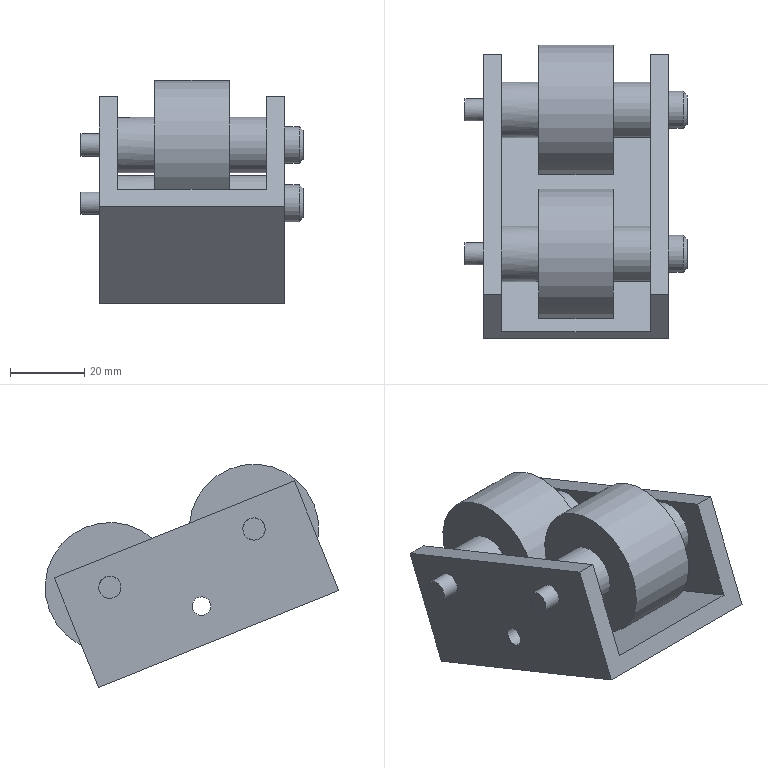Part | NX | features solid 2 | 1 solid | 32 faces | box 60 x 79.34 x 60.356 mm | volume 82796 mm3 | plane 18 | cylinder 12 | cone 2 | commonest cylinder face diameters 15 x4 5 x2 6 x2 10 x2 35 x2
STEP:
#1=CARTESIAN_POINT('',(-651.881,525.03,-99.486));
#2=VERTEX_POINT('',#1);
#3=CARTESIAN_POINT('',(-691.881,525.03,-99.486));
#4=VERTEX_POINT('',#3);
#5=CARTESIAN_POINT('',(-646.881,525.03,-99.486));
#6=DIRECTION('',(-1.,0.,0.));
#7=VECTOR('',#6,1000.);
#8=LINE('',#5,#7);
#9=EDGE_CURVE('',#2,#4,#8,.T.);
#10=ORIENTED_EDGE('',*,*,#9,.F.);
#11=CARTESIAN_POINT('',(-651.881,535.144,-74.452));
#12=VERTEX_POINT('',#11);
#13=CARTESIAN_POINT('',(-651.881,535.144,-74.452));
#14=DIRECTION('',(0.,-0.3746,-0.9272));
#15=VECTOR('',#14,1000.);
#16=LINE('',#13,#15);
#17=EDGE_CURVE('',#12,#2,#16,.T.);
#18=ORIENTED_EDGE('',*,*,#17,.F.);
#19=CARTESIAN_POINT('',(-646.881,535.144,-74.452));
#20=VERTEX_POINT('',#19);
#21=CARTESIAN_POINT('',(-646.881,535.144,-74.452));
#22=DIRECTION('',(-1.,0.,0.));
#23=VECTOR('',#22,1000.);
#24=LINE('',#21,#23);
#25=EDGE_CURVE('',#12,#20,#24,.F.);
#26=ORIENTED_EDGE('',*,*,#25,.T.);
#27=CARTESIAN_POINT('',(-646.881,523.157,-104.122));
#28=VERTEX_POINT('',#27);
#29=CARTESIAN_POINT('',(-646.881,535.144,-74.452));
#30=DIRECTION('',(0.,-0.3746,-0.9272));
#31=VECTOR('',#30,1000.);
#32=LINE('',#29,#31);
#33=EDGE_CURVE('',#20,#28,#32,.T.);
#34=ORIENTED_EDGE('',*,*,#33,.T.);
#35=CARTESIAN_POINT('',(-696.881,523.157,-104.122));
#36=VERTEX_POINT('',#35);
#37=CARTESIAN_POINT('',(-646.881,523.157,-104.122));
#38=DIRECTION('',(-1.,0.,0.));
#39=VECTOR('',#38,1000.);
#40=LINE('',#37,#39);
#41=EDGE_CURVE('',#28,#36,#40,.T.);
#42=ORIENTED_EDGE('',*,*,#41,.T.);
#43=CARTESIAN_POINT('',(-696.881,535.144,-74.452));
#44=VERTEX_POINT('',#43);
#45=CARTESIAN_POINT('',(-696.881,523.157,-104.122));
#46=DIRECTION('',(0.,0.3746,0.9272));
#47=VECTOR('',#46,1000.);
#48=LINE('',#45,#47);
#49=EDGE_CURVE('',#36,#44,#48,.T.);
#50=ORIENTED_EDGE('',*,*,#49,.T.);
#51=CARTESIAN_POINT('',(-691.881,535.144,-74.452));
#52=VERTEX_POINT('',#51);
#53=CARTESIAN_POINT('',(-696.881,535.144,-74.452));
#54=DIRECTION('',(1.,0.,0.));
#55=VECTOR('',#54,1000.);
#56=LINE('',#53,#55);
#57=EDGE_CURVE('',#44,#52,#56,.T.);
#58=ORIENTED_EDGE('',*,*,#57,.T.);
#59=CARTESIAN_POINT('',(-691.881,523.157,-104.122));
#60=DIRECTION('',(0.,0.3746,0.9272));
#61=VECTOR('',#60,1000.);
#62=LINE('',#59,#61);
#63=EDGE_CURVE('',#4,#52,#62,.T.);
#64=ORIENTED_EDGE('',*,*,#63,.F.);
#65=EDGE_LOOP('',(#10,#18,#26,#34,#42,#50,#58,#64));
#66=FACE_BOUND('',#65,.T.);
#67=CARTESIAN_POINT('',(-646.881,535.144,-74.452));
#68=DIRECTION('',(0.,-0.9272,0.3746));
#69=DIRECTION('',(0.,-0.3746,-0.9272));
#70=AXIS2_PLACEMENT_3D('',#67,#68,#69);
#71=PLANE('',#70);
#72=ADVANCED_FACE('',(#66),#71,.F.);
#73=CARTESIAN_POINT('',(-691.881,483.962,-54.313));
#74=VERTEX_POINT('',#73);
#75=CARTESIAN_POINT('',(-691.881,481.152,-61.267));
#76=DIRECTION('',(-1.,0.,0.));
#77=DIRECTION('',(0.,0.3746,0.9272));
#78=AXIS2_PLACEMENT_3D('',#75,#76,#77);
#79=CIRCLE('',#78,7.5);
#80=EDGE_CURVE('',#74,#74,#79,.F.);
#81=ORIENTED_EDGE('',*,*,#80,.F.);
#82=EDGE_LOOP('',(#81));
#83=FACE_BOUND('',#82,.T.);
#84=CARTESIAN_POINT('',(-691.881,460.127,-73.264));
#85=VERTEX_POINT('',#84);
#86=CARTESIAN_POINT('',(-691.881,460.127,-73.264));
#87=DIRECTION('',(0.,0.9272,-0.3746));
#88=VECTOR('',#87,1000.);
#89=LINE('',#86,#88);
#90=EDGE_CURVE('',#85,#4,#89,.T.);
#91=ORIENTED_EDGE('',*,*,#90,.T.);
#92=ORIENTED_EDGE('',*,*,#63,.T.);
#93=CARTESIAN_POINT('',(-691.881,470.241,-48.23));
#94=VERTEX_POINT('',#93);
#95=CARTESIAN_POINT('',(-691.881,470.241,-48.23));
#96=DIRECTION('',(0.,0.9272,-0.3746));
#97=VECTOR('',#96,1000.);
#98=LINE('',#95,#97);
#99=EDGE_CURVE('',#94,#52,#98,.T.);
#100=ORIENTED_EDGE('',*,*,#99,.F.);
#101=CARTESIAN_POINT('',(-691.881,458.254,-77.9));
#102=DIRECTION('',(0.,0.3746,0.9272));
#103=VECTOR('',#102,1000.);
#104=LINE('',#101,#103);
#105=EDGE_CURVE('',#85,#94,#104,.T.);
#106=ORIENTED_EDGE('',*,*,#105,.F.);
#107=EDGE_LOOP('',(#91,#92,#100,#106));
#108=FACE_BOUND('',#107,.T.);
#109=CARTESIAN_POINT('',(-691.881,496.315,-79.796));
#110=VERTEX_POINT('',#109);
#111=CARTESIAN_POINT('',(-691.881,495.379,-82.114));
#112=DIRECTION('',(-1.,0.,0.));
#113=DIRECTION('',(0.,0.3746,0.9272));
#114=AXIS2_PLACEMENT_3D('',#111,#112,#113);
#115=CIRCLE('',#114,2.5);
#116=EDGE_CURVE('',#110,#110,#115,.F.);
#117=ORIENTED_EDGE('',*,*,#116,.F.);
#118=EDGE_LOOP('',(#117));
#119=FACE_BOUND('',#118,.T.);
#120=CARTESIAN_POINT('',(-691.881,522.904,-70.046));
#121=VERTEX_POINT('',#120);
#122=CARTESIAN_POINT('',(-691.881,520.094,-77.));
#123=DIRECTION('',(-1.,0.,0.));
#124=DIRECTION('',(0.,0.3746,0.9272));
#125=AXIS2_PLACEMENT_3D('',#122,#123,#124);
#126=CIRCLE('',#125,7.5);
#127=EDGE_CURVE('',#121,#121,#126,.F.);
#128=ORIENTED_EDGE('',*,*,#127,.F.);
#129=EDGE_LOOP('',(#128));
#130=FACE_BOUND('',#129,.T.);
#131=CARTESIAN_POINT('',(-691.881,458.254,-77.9));
#132=DIRECTION('',(-1.,0.,0.));
#133=DIRECTION('',(0.,0.3746,0.9272));
#134=AXIS2_PLACEMENT_3D('',#131,#132,#133);
#135=PLANE('',#134);
#136=ADVANCED_FACE('',(#83,#108,#119,#130),#135,.F.);
#137=CARTESIAN_POINT('',(-651.881,527.048,-79.81));
#138=VERTEX_POINT('',#137);
#139=CARTESIAN_POINT('',(-651.881,520.094,-77.));
#140=DIRECTION('',(-1.,0.,0.));
#141=DIRECTION('',(0.,0.9272,-0.3746));
#142=AXIS2_PLACEMENT_3D('',#139,#140,#141);
#143=CIRCLE('',#142,7.5);
#144=EDGE_CURVE('',#138,#138,#143,.T.);
#145=ORIENTED_EDGE('',*,*,#144,.F.);
#146=EDGE_LOOP('',(#145));
#147=FACE_BOUND('',#146,.T.);
#148=CARTESIAN_POINT('',(-651.881,494.442,-84.432));
#149=VERTEX_POINT('',#148);
#150=CARTESIAN_POINT('',(-651.881,495.379,-82.114));
#151=DIRECTION('',(1.,0.,0.));
#152=DIRECTION('',(0.,-0.3746,-0.9272));
#153=AXIS2_PLACEMENT_3D('',#150,#151,#152);
#154=CIRCLE('',#153,2.5);
#155=EDGE_CURVE('',#149,#149,#154,.F.);
#156=ORIENTED_EDGE('',*,*,#155,.F.);
#157=EDGE_LOOP('',(#156));
#158=FACE_BOUND('',#157,.T.);
#159=CARTESIAN_POINT('',(-651.881,488.106,-64.076));
#160=VERTEX_POINT('',#159);
#161=CARTESIAN_POINT('',(-651.881,481.152,-61.267));
#162=DIRECTION('',(-1.,0.,0.));
#163=DIRECTION('',(0.,0.9272,-0.3746));
#164=AXIS2_PLACEMENT_3D('',#161,#162,#163);
#165=CIRCLE('',#164,7.5);
#166=EDGE_CURVE('',#160,#160,#165,.T.);
#167=ORIENTED_EDGE('',*,*,#166,.F.);
#168=EDGE_LOOP('',(#167));
#169=FACE_BOUND('',#168,.T.);
#170=CARTESIAN_POINT('',(-651.881,470.241,-48.23));
#171=VERTEX_POINT('',#170);
#172=CARTESIAN_POINT('',(-651.881,470.241,-48.23));
#173=DIRECTION('',(0.,0.9272,-0.3746));
#174=VECTOR('',#173,1000.);
#175=LINE('',#172,#174);
#176=EDGE_CURVE('',#171,#12,#175,.T.);
#177=ORIENTED_EDGE('',*,*,#176,.T.);
#178=ORIENTED_EDGE('',*,*,#17,.T.);
#179=CARTESIAN_POINT('',(-651.881,460.127,-73.264));
#180=VERTEX_POINT('',#179);
#181=CARTESIAN_POINT('',(-651.881,460.127,-73.264));
#182=DIRECTION('',(0.,0.9272,-0.3746));
#183=VECTOR('',#182,1000.);
#184=LINE('',#181,#183);
#185=EDGE_CURVE('',#180,#2,#184,.T.);
#186=ORIENTED_EDGE('',*,*,#185,.F.);
#187=CARTESIAN_POINT('',(-651.881,470.241,-48.23));
#188=DIRECTION('',(0.,-0.3746,-0.9272));
#189=VECTOR('',#188,1000.);
#190=LINE('',#187,#189);
#191=EDGE_CURVE('',#171,#180,#190,.T.);
#192=ORIENTED_EDGE('',*,*,#191,.F.);
#193=EDGE_LOOP('',(#177,#178,#186,#192));
#194=FACE_BOUND('',#193,.T.);
#195=CARTESIAN_POINT('',(-651.881,470.241,-48.23));
#196=DIRECTION('',(1.,0.,0.));
#197=DIRECTION('',(0.,-0.3746,-0.9272));
#198=AXIS2_PLACEMENT_3D('',#195,#196,#197);
#199=PLANE('',#198);
#200=ADVANCED_FACE('',(#147,#158,#169,#194),#199,.F.);
#201=ORIENTED_EDGE('',*,*,#49,.F.);
#202=CARTESIAN_POINT('',(-696.881,458.254,-77.9));
#203=VERTEX_POINT('',#202);
#204=CARTESIAN_POINT('',(-696.881,458.254,-77.9));
#205=DIRECTION('',(0.,0.9272,-0.3746));
#206=VECTOR('',#205,1000.);
#207=LINE('',#204,#206);
#208=EDGE_CURVE('',#203,#36,#207,.T.);
#209=ORIENTED_EDGE('',*,*,#208,.F.);
#210=CARTESIAN_POINT('',(-696.881,470.241,-48.23));
#211=VERTEX_POINT('',#210);
#212=CARTESIAN_POINT('',(-696.881,458.254,-77.9));
#213=DIRECTION('',(0.,0.3746,0.9272));
#214=VECTOR('',#213,1000.);
#215=LINE('',#212,#214);
#216=EDGE_CURVE('',#203,#211,#215,.T.);
#217=ORIENTED_EDGE('',*,*,#216,.T.);
#218=CARTESIAN_POINT('',(-696.881,470.241,-48.23));
#219=DIRECTION('',(0.,0.9272,-0.3746));
#220=VECTOR('',#219,1000.);
#221=LINE('',#218,#220);
#222=EDGE_CURVE('',#211,#44,#221,.T.);
#223=ORIENTED_EDGE('',*,*,#222,.T.);
#224=EDGE_LOOP('',(#201,#209,#217,#223));
#225=FACE_BOUND('',#224,.T.);
#226=CARTESIAN_POINT('',(-696.881,496.315,-79.796));
#227=VERTEX_POINT('',#226);
#228=CARTESIAN_POINT('',(-696.881,495.379,-82.114));
#229=DIRECTION('',(-1.,0.,0.));
#230=DIRECTION('',(0.,0.3746,0.9272));
#231=AXIS2_PLACEMENT_3D('',#228,#229,#230);
#232=CIRCLE('',#231,2.5);
#233=EDGE_CURVE('',#227,#227,#232,.F.);
#234=ORIENTED_EDGE('',*,*,#233,.T.);
#235=EDGE_LOOP('',(#234));
#236=FACE_BOUND('',#235,.T.);
#237=CARTESIAN_POINT('',(-696.881,482.276,-58.485));
#238=VERTEX_POINT('',#237);
#239=CARTESIAN_POINT('',(-696.881,481.152,-61.267));
#240=DIRECTION('',(-1.,0.,0.));
#241=DIRECTION('',(0.,0.3746,0.9272));
#242=AXIS2_PLACEMENT_3D('',#239,#240,#241);
#243=CIRCLE('',#242,3.);
#244=EDGE_CURVE('',#238,#238,#243,.F.);
#245=ORIENTED_EDGE('',*,*,#244,.T.);
#246=EDGE_LOOP('',(#245));
#247=FACE_BOUND('',#246,.T.);
#248=CARTESIAN_POINT('',(-696.881,521.218,-74.218));
#249=VERTEX_POINT('',#248);
#250=CARTESIAN_POINT('',(-696.881,520.094,-77.));
#251=DIRECTION('',(-1.,0.,0.));
#252=DIRECTION('',(0.,0.3746,0.9272));
#253=AXIS2_PLACEMENT_3D('',#250,#251,#252);
#254=CIRCLE('',#253,3.);
#255=EDGE_CURVE('',#249,#249,#254,.F.);
#256=ORIENTED_EDGE('',*,*,#255,.T.);
#257=EDGE_LOOP('',(#256));
#258=FACE_BOUND('',#257,.T.);
#259=CARTESIAN_POINT('',(-696.881,458.254,-77.9));
#260=DIRECTION('',(-1.,0.,0.));
#261=DIRECTION('',(0.,0.3746,0.9272));
#262=AXIS2_PLACEMENT_3D('',#259,#260,#261);
#263=PLANE('',#262);
#264=ADVANCED_FACE('',(#225,#236,#247,#258),#263,.T.);
#265=ORIENTED_EDGE('',*,*,#33,.F.);
#266=CARTESIAN_POINT('',(-646.881,470.241,-48.23));
#267=VERTEX_POINT('',#266);
#268=CARTESIAN_POINT('',(-646.881,470.241,-48.23));
#269=DIRECTION('',(0.,0.9272,-0.3746));
#270=VECTOR('',#269,1000.);
#271=LINE('',#268,#270);
#272=EDGE_CURVE('',#267,#20,#271,.T.);
#273=ORIENTED_EDGE('',*,*,#272,.F.);
#274=CARTESIAN_POINT('',(-646.881,458.254,-77.9));
#275=VERTEX_POINT('',#274);
#276=CARTESIAN_POINT('',(-646.881,470.241,-48.23));
#277=DIRECTION('',(0.,-0.3746,-0.9272));
#278=VECTOR('',#277,1000.);
#279=LINE('',#276,#278);
#280=EDGE_CURVE('',#267,#275,#279,.T.);
#281=ORIENTED_EDGE('',*,*,#280,.T.);
#282=CARTESIAN_POINT('',(-646.881,458.254,-77.9));
#283=DIRECTION('',(0.,0.9272,-0.3746));
#284=VECTOR('',#283,1000.);
#285=LINE('',#282,#284);
#286=EDGE_CURVE('',#275,#28,#285,.T.);
#287=ORIENTED_EDGE('',*,*,#286,.T.);
#288=EDGE_LOOP('',(#265,#273,#281,#287));
#289=FACE_BOUND('',#288,.T.);
#290=CARTESIAN_POINT('',(-646.881,518.221,-81.636));
#291=VERTEX_POINT('',#290);
#292=CARTESIAN_POINT('',(-646.881,520.094,-77.));
#293=DIRECTION('',(1.,0.,0.));
#294=DIRECTION('',(0.,-0.3746,-0.9272));
#295=AXIS2_PLACEMENT_3D('',#292,#293,#294);
#296=CIRCLE('',#295,5.);
#297=EDGE_CURVE('',#291,#291,#296,.T.);
#298=ORIENTED_EDGE('',*,*,#297,.F.);
#299=EDGE_LOOP('',(#298));
#300=FACE_BOUND('',#299,.T.);
#301=CARTESIAN_POINT('',(-646.881,494.442,-84.432));
#302=VERTEX_POINT('',#301);
#303=CARTESIAN_POINT('',(-646.881,495.379,-82.114));
#304=DIRECTION('',(1.,0.,0.));
#305=DIRECTION('',(0.,-0.3746,-0.9272));
#306=AXIS2_PLACEMENT_3D('',#303,#304,#305);
#307=CIRCLE('',#306,2.5);
#308=EDGE_CURVE('',#302,#302,#307,.F.);
#309=ORIENTED_EDGE('',*,*,#308,.T.);
#310=EDGE_LOOP('',(#309));
#311=FACE_BOUND('',#310,.T.);
#312=CARTESIAN_POINT('',(-646.881,479.279,-65.902));
#313=VERTEX_POINT('',#312);
#314=CARTESIAN_POINT('',(-646.881,481.152,-61.267));
#315=DIRECTION('',(1.,0.,0.));
#316=DIRECTION('',(0.,-0.3746,-0.9272));
#317=AXIS2_PLACEMENT_3D('',#314,#315,#316);
#318=CIRCLE('',#317,5.);
#319=EDGE_CURVE('',#313,#313,#318,.T.);
#320=ORIENTED_EDGE('',*,*,#319,.F.);
#321=EDGE_LOOP('',(#320));
#322=FACE_BOUND('',#321,.T.);
#323=CARTESIAN_POINT('',(-646.881,470.241,-48.23));
#324=DIRECTION('',(1.,0.,0.));
#325=DIRECTION('',(0.,-0.3746,-0.9272));
#326=AXIS2_PLACEMENT_3D('',#323,#324,#325);
#327=PLANE('',#326);
#328=ADVANCED_FACE('',(#289,#300,#311,#322),#327,.T.);
#329=CARTESIAN_POINT('',(-681.881,536.32,-83.556));
#330=VERTEX_POINT('',#329);
#331=CARTESIAN_POINT('',(-681.881,520.094,-77.));
#332=DIRECTION('',(-1.,0.,0.));
#333=DIRECTION('',(0.,0.9272,-0.3746));
#334=AXIS2_PLACEMENT_3D('',#331,#332,#333);
#335=CIRCLE('',#334,17.5);
#336=EDGE_CURVE('',#330,#330,#335,.T.);
#337=ORIENTED_EDGE('',*,*,#336,.T.);
#338=EDGE_LOOP('',(#337));
#339=FACE_BOUND('',#338,.T.);
#340=CARTESIAN_POINT('',(-681.881,527.048,-79.81));
#341=VERTEX_POINT('',#340);
#342=CARTESIAN_POINT('',(-681.881,520.094,-77.));
#343=DIRECTION('',(-1.,0.,0.));
#344=DIRECTION('',(0.,0.9272,-0.3746));
#345=AXIS2_PLACEMENT_3D('',#342,#343,#344);
#346=CIRCLE('',#345,7.5);
#347=EDGE_CURVE('',#341,#341,#346,.T.);
#348=ORIENTED_EDGE('',*,*,#347,.F.);
#349=EDGE_LOOP('',(#348));
#350=FACE_BOUND('',#349,.T.);
#351=CARTESIAN_POINT('',(-681.881,520.094,-77.));
#352=DIRECTION('',(-1.,0.,0.));
#353=DIRECTION('',(0.,0.3746,0.9272));
#354=AXIS2_PLACEMENT_3D('',#351,#352,#353);
#355=PLANE('',#354);
#356=ADVANCED_FACE('',(#339,#350),#355,.T.);
#357=CARTESIAN_POINT('',(-681.881,497.378,-67.822));
#358=VERTEX_POINT('',#357);
#359=CARTESIAN_POINT('',(-681.881,481.152,-61.267));
#360=DIRECTION('',(-1.,0.,0.));
#361=DIRECTION('',(0.,0.9272,-0.3746));
#362=AXIS2_PLACEMENT_3D('',#359,#360,#361);
#363=CIRCLE('',#362,17.5);
#364=EDGE_CURVE('',#358,#358,#363,.T.);
#365=ORIENTED_EDGE('',*,*,#364,.T.);
#366=EDGE_LOOP('',(#365));
#367=FACE_BOUND('',#366,.T.);
#368=CARTESIAN_POINT('',(-681.881,488.106,-64.076));
#369=VERTEX_POINT('',#368);
#370=CARTESIAN_POINT('',(-681.881,481.152,-61.267));
#371=DIRECTION('',(-1.,0.,0.));
#372=DIRECTION('',(0.,0.9272,-0.3746));
#373=AXIS2_PLACEMENT_3D('',#370,#371,#372);
#374=CIRCLE('',#373,7.5);
#375=EDGE_CURVE('',#369,#369,#374,.T.);
#376=ORIENTED_EDGE('',*,*,#375,.F.);
#377=EDGE_LOOP('',(#376));
#378=FACE_BOUND('',#377,.T.);
#379=CARTESIAN_POINT('',(-681.881,481.152,-61.267));
#380=DIRECTION('',(-1.,0.,0.));
#381=DIRECTION('',(0.,0.3746,0.9272));
#382=AXIS2_PLACEMENT_3D('',#379,#380,#381);
#383=PLANE('',#382);
#384=ADVANCED_FACE('',(#367,#378),#383,.T.);
#385=ORIENTED_EDGE('',*,*,#191,.T.);
#386=CARTESIAN_POINT('',(-646.881,460.127,-73.264));
#387=DIRECTION('',(-1.,0.,0.));
#388=VECTOR('',#387,1000.);
#389=LINE('',#386,#388);
#390=EDGE_CURVE('',#180,#85,#389,.T.);
#391=ORIENTED_EDGE('',*,*,#390,.T.);
#392=ORIENTED_EDGE('',*,*,#105,.T.);
#393=CARTESIAN_POINT('',(-696.881,470.241,-48.23));
#394=DIRECTION('',(1.,0.,0.));
#395=VECTOR('',#394,1000.);
#396=LINE('',#393,#395);
#397=EDGE_CURVE('',#211,#94,#396,.T.);
#398=ORIENTED_EDGE('',*,*,#397,.F.);
#399=ORIENTED_EDGE('',*,*,#216,.F.);
#400=CARTESIAN_POINT('',(-646.881,458.254,-77.9));
#401=DIRECTION('',(-1.,0.,0.));
#402=VECTOR('',#401,1000.);
#403=LINE('',#400,#402);
#404=EDGE_CURVE('',#275,#203,#403,.T.);
#405=ORIENTED_EDGE('',*,*,#404,.F.);
#406=ORIENTED_EDGE('',*,*,#280,.F.);
#407=CARTESIAN_POINT('',(-646.881,470.241,-48.23));
#408=DIRECTION('',(-1.,0.,0.));
#409=VECTOR('',#408,1000.);
#410=LINE('',#407,#409);
#411=EDGE_CURVE('',#267,#171,#410,.T.);
#412=ORIENTED_EDGE('',*,*,#411,.T.);
#413=EDGE_LOOP('',(#385,#391,#392,#398,#399,#405,#406,#412));
#414=FACE_BOUND('',#413,.T.);
#415=CARTESIAN_POINT('',(-646.881,470.241,-48.23));
#416=DIRECTION('',(0.,-0.9272,0.3746));
#417=DIRECTION('',(0.,-0.3746,-0.9272));
#418=AXIS2_PLACEMENT_3D('',#415,#416,#417);
#419=PLANE('',#418);
#420=ADVANCED_FACE('',(#414),#419,.T.);
#421=ORIENTED_EDGE('',*,*,#25,.F.);
#422=ORIENTED_EDGE('',*,*,#176,.F.);
#423=ORIENTED_EDGE('',*,*,#411,.F.);
#424=ORIENTED_EDGE('',*,*,#272,.T.);
#425=EDGE_LOOP('',(#421,#422,#423,#424));
#426=FACE_BOUND('',#425,.T.);
#427=CARTESIAN_POINT('',(-646.881,470.241,-48.23));
#428=DIRECTION('',(0.,-0.3746,-0.9272));
#429=DIRECTION('',(0.,0.9272,-0.3746));
#430=AXIS2_PLACEMENT_3D('',#427,#428,#429);
#431=PLANE('',#430);
#432=ADVANCED_FACE('',(#426),#431,.F.);
#433=ORIENTED_EDGE('',*,*,#185,.T.);
#434=ORIENTED_EDGE('',*,*,#9,.T.);
#435=ORIENTED_EDGE('',*,*,#90,.F.);
#436=ORIENTED_EDGE('',*,*,#390,.F.);
#437=EDGE_LOOP('',(#433,#434,#435,#436));
#438=FACE_BOUND('',#437,.T.);
#439=CARTESIAN_POINT('',(-646.881,460.127,-73.264));
#440=DIRECTION('',(0.,-0.3746,-0.9272));
#441=DIRECTION('',(0.,-0.9272,0.3746));
#442=AXIS2_PLACEMENT_3D('',#439,#440,#441);
#443=PLANE('',#442);
#444=ADVANCED_FACE('',(#438),#443,.F.);
#445=ORIENTED_EDGE('',*,*,#57,.F.);
#446=ORIENTED_EDGE('',*,*,#222,.F.);
#447=ORIENTED_EDGE('',*,*,#397,.T.);
#448=ORIENTED_EDGE('',*,*,#99,.T.);
#449=EDGE_LOOP('',(#445,#446,#447,#448));
#450=FACE_BOUND('',#449,.T.);
#451=CARTESIAN_POINT('',(-696.881,470.241,-48.23));
#452=DIRECTION('',(0.,0.3746,0.9272));
#453=DIRECTION('',(0.,0.9272,-0.3746));
#454=AXIS2_PLACEMENT_3D('',#451,#452,#453);
#455=PLANE('',#454);
#456=ADVANCED_FACE('',(#450),#455,.T.);
#457=ORIENTED_EDGE('',*,*,#41,.F.);
#458=ORIENTED_EDGE('',*,*,#286,.F.);
#459=ORIENTED_EDGE('',*,*,#404,.T.);
#460=ORIENTED_EDGE('',*,*,#208,.T.);
#461=EDGE_LOOP('',(#457,#458,#459,#460));
#462=FACE_BOUND('',#461,.T.);
#463=CARTESIAN_POINT('',(-646.881,458.254,-77.9));
#464=DIRECTION('',(0.,-0.3746,-0.9272));
#465=DIRECTION('',(0.,-0.9272,0.3746));
#466=AXIS2_PLACEMENT_3D('',#463,#464,#465);
#467=PLANE('',#466);
#468=ADVANCED_FACE('',(#462),#467,.T.);
#469=CARTESIAN_POINT('',(-701.881,483.934,-62.39));
#470=VERTEX_POINT('',#469);
#471=CARTESIAN_POINT('',(-701.881,481.152,-61.267));
#472=DIRECTION('',(-1.,0.,0.));
#473=DIRECTION('',(0.,0.9272,-0.3746));
#474=AXIS2_PLACEMENT_3D('',#471,#472,#473);
#475=CIRCLE('',#474,3.);
#476=EDGE_CURVE('',#470,#470,#475,.T.);
#477=ORIENTED_EDGE('',*,*,#476,.T.);
#478=EDGE_LOOP('',(#477));
#479=FACE_BOUND('',#478,.T.);
#480=CARTESIAN_POINT('',(-701.881,481.152,-61.267));
#481=DIRECTION('',(-1.,0.,0.));
#482=DIRECTION('',(0.,0.3746,0.9272));
#483=AXIS2_PLACEMENT_3D('',#480,#481,#482);
#484=PLANE('',#483);
#485=ADVANCED_FACE('',(#479),#484,.T.);
#486=ORIENTED_EDGE('',*,*,#244,.F.);
#487=EDGE_LOOP('',(#486));
#488=FACE_BOUND('',#487,.T.);
#489=ORIENTED_EDGE('',*,*,#476,.F.);
#490=EDGE_LOOP('',(#489));
#491=FACE_BOUND('',#490,.T.);
#492=CARTESIAN_POINT('',(-701.881,481.152,-61.267));
#493=DIRECTION('',(1.,0.,0.));
#494=DIRECTION('',(0.,-0.3746,-0.9272));
#495=AXIS2_PLACEMENT_3D('',#492,#493,#494);
#496=CYLINDRICAL_SURFACE('',#495,3.);
#497=ADVANCED_FACE('',(#488,#491),#496,.T.);
#498=CARTESIAN_POINT('',(-661.881,488.106,-64.076));
#499=VERTEX_POINT('',#498);
#500=CARTESIAN_POINT('',(-661.881,481.152,-61.267));
#501=DIRECTION('',(-1.,0.,0.));
#502=DIRECTION('',(0.,0.9272,-0.3746));
#503=AXIS2_PLACEMENT_3D('',#500,#501,#502);
#504=CIRCLE('',#503,7.5);
#505=EDGE_CURVE('',#499,#499,#504,.T.);
#506=ORIENTED_EDGE('',*,*,#505,.T.);
#507=EDGE_LOOP('',(#506));
#508=FACE_BOUND('',#507,.T.);
#509=CARTESIAN_POINT('',(-661.881,497.378,-67.822));
#510=VERTEX_POINT('',#509);
#511=CARTESIAN_POINT('',(-661.881,481.152,-61.267));
#512=DIRECTION('',(-1.,0.,0.));
#513=DIRECTION('',(0.,0.9272,-0.3746));
#514=AXIS2_PLACEMENT_3D('',#511,#512,#513);
#515=CIRCLE('',#514,17.5);
#516=EDGE_CURVE('',#510,#510,#515,.T.);
#517=ORIENTED_EDGE('',*,*,#516,.F.);
#518=EDGE_LOOP('',(#517));
#519=FACE_BOUND('',#518,.T.);
#520=CARTESIAN_POINT('',(-661.881,481.152,-61.267));
#521=DIRECTION('',(-1.,0.,0.));
#522=DIRECTION('',(0.,0.3746,0.9272));
#523=AXIS2_PLACEMENT_3D('',#520,#521,#522);
#524=PLANE('',#523);
#525=ADVANCED_FACE('',(#508,#519),#524,.F.);
#526=ORIENTED_EDGE('',*,*,#364,.F.);
#527=EDGE_LOOP('',(#526));
#528=FACE_BOUND('',#527,.T.);
#529=ORIENTED_EDGE('',*,*,#516,.T.);
#530=EDGE_LOOP('',(#529));
#531=FACE_BOUND('',#530,.T.);
#532=CARTESIAN_POINT('',(-681.881,481.152,-61.267));
#533=DIRECTION('',(1.,0.,0.));
#534=DIRECTION('',(0.,-0.3746,-0.9272));
#535=AXIS2_PLACEMENT_3D('',#532,#533,#534);
#536=CYLINDRICAL_SURFACE('',#535,17.5);
#537=ADVANCED_FACE('',(#528,#531),#536,.T.);
#538=ORIENTED_EDGE('',*,*,#80,.T.);
#539=EDGE_LOOP('',(#538));
#540=FACE_BOUND('',#539,.T.);
#541=ORIENTED_EDGE('',*,*,#375,.T.);
#542=EDGE_LOOP('',(#541));
#543=FACE_BOUND('',#542,.T.);
#544=CARTESIAN_POINT('',(-691.881,481.152,-61.267));
#545=DIRECTION('',(1.,0.,0.));
#546=DIRECTION('',(0.,-0.3746,-0.9272));
#547=AXIS2_PLACEMENT_3D('',#544,#545,#546);
#548=CYLINDRICAL_SURFACE('',#547,7.5);
#549=ADVANCED_FACE('',(#540,#543),#548,.T.);
#550=ORIENTED_EDGE('',*,*,#166,.T.);
#551=EDGE_LOOP('',(#550));
#552=FACE_BOUND('',#551,.T.);
#553=ORIENTED_EDGE('',*,*,#505,.F.);
#554=EDGE_LOOP('',(#553));
#555=FACE_BOUND('',#554,.T.);
#556=CARTESIAN_POINT('',(-651.881,481.152,-61.267));
#557=DIRECTION('',(-1.,0.,0.));
#558=DIRECTION('',(0.,0.3746,0.9272));
#559=AXIS2_PLACEMENT_3D('',#556,#557,#558);
#560=CYLINDRICAL_SURFACE('',#559,7.5);
#561=ADVANCED_FACE('',(#552,#555),#560,.T.);
#562=CARTESIAN_POINT('',(-642.881,483.025,-56.631));
#563=VERTEX_POINT('',#562);
#564=CARTESIAN_POINT('',(-642.881,481.152,-61.267));
#565=DIRECTION('',(-1.,0.,0.));
#566=DIRECTION('',(0.,0.3746,0.9272));
#567=AXIS2_PLACEMENT_3D('',#564,#565,#566);
#568=CIRCLE('',#567,5.);
#569=EDGE_CURVE('',#563,#563,#568,.T.);
#570=ORIENTED_EDGE('',*,*,#569,.T.);
#571=EDGE_LOOP('',(#570));
#572=FACE_BOUND('',#571,.T.);
#573=ORIENTED_EDGE('',*,*,#319,.T.);
#574=EDGE_LOOP('',(#573));
#575=FACE_BOUND('',#574,.T.);
#576=CARTESIAN_POINT('',(-641.881,481.152,-61.267));
#577=DIRECTION('',(-1.,0.,0.));
#578=DIRECTION('',(0.,0.3746,0.9272));
#579=AXIS2_PLACEMENT_3D('',#576,#577,#578);
#580=CYLINDRICAL_SURFACE('',#579,5.);
#581=ADVANCED_FACE('',(#572,#575),#580,.T.);
#582=CARTESIAN_POINT('',(-641.881,482.651,-57.558));
#583=VERTEX_POINT('',#582);
#584=CARTESIAN_POINT('',(-641.881,481.152,-61.267));
#585=DIRECTION('',(-1.,0.,0.));
#586=DIRECTION('',(0.,0.3746,0.9272));
#587=AXIS2_PLACEMENT_3D('',#584,#585,#586);
#588=CIRCLE('',#587,4.);
#589=EDGE_CURVE('',#583,#583,#588,.F.);
#590=ORIENTED_EDGE('',*,*,#589,.T.);
#591=EDGE_LOOP('',(#590));
#592=FACE_BOUND('',#591,.T.);
#593=CARTESIAN_POINT('',(-641.881,481.152,-61.267));
#594=DIRECTION('',(-1.,0.,0.));
#595=DIRECTION('',(0.,0.3746,0.9272));
#596=AXIS2_PLACEMENT_3D('',#593,#594,#595);
#597=PLANE('',#596);
#598=ADVANCED_FACE('',(#592),#597,.F.);
#599=ORIENTED_EDGE('',*,*,#308,.F.);
#600=EDGE_LOOP('',(#599));
#601=FACE_BOUND('',#600,.T.);
#602=ORIENTED_EDGE('',*,*,#155,.T.);
#603=EDGE_LOOP('',(#602));
#604=FACE_BOUND('',#603,.T.);
#605=CARTESIAN_POINT('',(-701.881,495.379,-82.114));
#606=DIRECTION('',(1.,0.,0.));
#607=DIRECTION('',(0.,-0.3746,-0.9272));
#608=AXIS2_PLACEMENT_3D('',#605,#606,#607);
#609=CYLINDRICAL_SURFACE('',#608,2.5);
#610=ADVANCED_FACE('',(#601,#604),#609,.F.);
#611=ORIENTED_EDGE('',*,*,#233,.F.);
#612=EDGE_LOOP('',(#611));
#613=FACE_BOUND('',#612,.T.);
#614=ORIENTED_EDGE('',*,*,#116,.T.);
#615=EDGE_LOOP('',(#614));
#616=FACE_BOUND('',#615,.T.);
#617=CARTESIAN_POINT('',(-701.881,495.379,-82.114));
#618=DIRECTION('',(1.,0.,0.));
#619=DIRECTION('',(0.,-0.3746,-0.9272));
#620=AXIS2_PLACEMENT_3D('',#617,#618,#619);
#621=CYLINDRICAL_SURFACE('',#620,2.5);
#622=ADVANCED_FACE('',(#613,#616),#621,.F.);
#623=CARTESIAN_POINT('',(-701.881,522.876,-78.124));
#624=VERTEX_POINT('',#623);
#625=CARTESIAN_POINT('',(-701.881,520.094,-77.));
#626=DIRECTION('',(-1.,0.,0.));
#627=DIRECTION('',(0.,0.9272,-0.3746));
#628=AXIS2_PLACEMENT_3D('',#625,#626,#627);
#629=CIRCLE('',#628,3.);
#630=EDGE_CURVE('',#624,#624,#629,.T.);
#631=ORIENTED_EDGE('',*,*,#630,.T.);
#632=EDGE_LOOP('',(#631));
#633=FACE_BOUND('',#632,.T.);
#634=CARTESIAN_POINT('',(-701.881,520.094,-77.));
#635=DIRECTION('',(-1.,0.,0.));
#636=DIRECTION('',(0.,0.3746,0.9272));
#637=AXIS2_PLACEMENT_3D('',#634,#635,#636);
#638=PLANE('',#637);
#639=ADVANCED_FACE('',(#633),#638,.T.);
#640=ORIENTED_EDGE('',*,*,#255,.F.);
#641=EDGE_LOOP('',(#640));
#642=FACE_BOUND('',#641,.T.);
#643=ORIENTED_EDGE('',*,*,#630,.F.);
#644=EDGE_LOOP('',(#643));
#645=FACE_BOUND('',#644,.T.);
#646=CARTESIAN_POINT('',(-701.881,520.094,-77.));
#647=DIRECTION('',(1.,0.,0.));
#648=DIRECTION('',(0.,-0.3746,-0.9272));
#649=AXIS2_PLACEMENT_3D('',#646,#647,#648);
#650=CYLINDRICAL_SURFACE('',#649,3.);
#651=ADVANCED_FACE('',(#642,#645),#650,.T.);
#652=CARTESIAN_POINT('',(-661.881,527.048,-79.81));
#653=VERTEX_POINT('',#652);
#654=CARTESIAN_POINT('',(-661.881,520.094,-77.));
#655=DIRECTION('',(-1.,0.,0.));
#656=DIRECTION('',(0.,0.9272,-0.3746));
#657=AXIS2_PLACEMENT_3D('',#654,#655,#656);
#658=CIRCLE('',#657,7.5);
#659=EDGE_CURVE('',#653,#653,#658,.T.);
#660=ORIENTED_EDGE('',*,*,#659,.T.);
#661=EDGE_LOOP('',(#660));
#662=FACE_BOUND('',#661,.T.);
#663=CARTESIAN_POINT('',(-661.881,536.32,-83.556));
#664=VERTEX_POINT('',#663);
#665=CARTESIAN_POINT('',(-661.881,520.094,-77.));
#666=DIRECTION('',(-1.,0.,0.));
#667=DIRECTION('',(0.,0.9272,-0.3746));
#668=AXIS2_PLACEMENT_3D('',#665,#666,#667);
#669=CIRCLE('',#668,17.5);
#670=EDGE_CURVE('',#664,#664,#669,.T.);
#671=ORIENTED_EDGE('',*,*,#670,.F.);
#672=EDGE_LOOP('',(#671));
#673=FACE_BOUND('',#672,.T.);
#674=CARTESIAN_POINT('',(-661.881,520.094,-77.));
#675=DIRECTION('',(-1.,0.,0.));
#676=DIRECTION('',(0.,0.3746,0.9272));
#677=AXIS2_PLACEMENT_3D('',#674,#675,#676);
#678=PLANE('',#677);
#679=ADVANCED_FACE('',(#662,#673),#678,.F.);
#680=ORIENTED_EDGE('',*,*,#336,.F.);
#681=EDGE_LOOP('',(#680));
#682=FACE_BOUND('',#681,.T.);
#683=ORIENTED_EDGE('',*,*,#670,.T.);
#684=EDGE_LOOP('',(#683));
#685=FACE_BOUND('',#684,.T.);
#686=CARTESIAN_POINT('',(-681.881,520.094,-77.));
#687=DIRECTION('',(1.,0.,0.));
#688=DIRECTION('',(0.,-0.3746,-0.9272));
#689=AXIS2_PLACEMENT_3D('',#686,#687,#688);
#690=CYLINDRICAL_SURFACE('',#689,17.5);
#691=ADVANCED_FACE('',(#682,#685),#690,.T.);
#692=ORIENTED_EDGE('',*,*,#127,.T.);
#693=EDGE_LOOP('',(#692));
#694=FACE_BOUND('',#693,.T.);
#695=ORIENTED_EDGE('',*,*,#347,.T.);
#696=EDGE_LOOP('',(#695));
#697=FACE_BOUND('',#696,.T.);
#698=CARTESIAN_POINT('',(-691.881,520.094,-77.));
#699=DIRECTION('',(1.,0.,0.));
#700=DIRECTION('',(0.,-0.3746,-0.9272));
#701=AXIS2_PLACEMENT_3D('',#698,#699,#700);
#702=CYLINDRICAL_SURFACE('',#701,7.5);
#703=ADVANCED_FACE('',(#694,#697),#702,.T.);
#704=ORIENTED_EDGE('',*,*,#144,.T.);
#705=EDGE_LOOP('',(#704));
#706=FACE_BOUND('',#705,.T.);
#707=ORIENTED_EDGE('',*,*,#659,.F.);
#708=EDGE_LOOP('',(#707));
#709=FACE_BOUND('',#708,.T.);
#710=CARTESIAN_POINT('',(-651.881,520.094,-77.));
#711=DIRECTION('',(-1.,0.,0.));
#712=DIRECTION('',(0.,0.3746,0.9272));
#713=AXIS2_PLACEMENT_3D('',#710,#711,#712);
#714=CYLINDRICAL_SURFACE('',#713,7.5);
#715=ADVANCED_FACE('',(#706,#709),#714,.T.);
#716=CARTESIAN_POINT('',(-642.881,521.967,-72.364));
#717=VERTEX_POINT('',#716);
#718=CARTESIAN_POINT('',(-642.881,520.094,-77.));
#719=DIRECTION('',(-1.,0.,0.));
#720=DIRECTION('',(0.,0.3746,0.9272));
#721=AXIS2_PLACEMENT_3D('',#718,#719,#720);
#722=CIRCLE('',#721,5.);
#723=EDGE_CURVE('',#717,#717,#722,.T.);
#724=ORIENTED_EDGE('',*,*,#723,.T.);
#725=EDGE_LOOP('',(#724));
#726=FACE_BOUND('',#725,.T.);
#727=ORIENTED_EDGE('',*,*,#297,.T.);
#728=EDGE_LOOP('',(#727));
#729=FACE_BOUND('',#728,.T.);
#730=CARTESIAN_POINT('',(-641.881,520.094,-77.));
#731=DIRECTION('',(-1.,0.,0.));
#732=DIRECTION('',(0.,0.3746,0.9272));
#733=AXIS2_PLACEMENT_3D('',#730,#731,#732);
#734=CYLINDRICAL_SURFACE('',#733,5.);
#735=ADVANCED_FACE('',(#726,#729),#734,.T.);
#736=CARTESIAN_POINT('',(-641.881,521.592,-73.291));
#737=VERTEX_POINT('',#736);
#738=CARTESIAN_POINT('',(-641.881,520.094,-77.));
#739=DIRECTION('',(-1.,0.,0.));
#740=DIRECTION('',(0.,0.3746,0.9272));
#741=AXIS2_PLACEMENT_3D('',#738,#739,#740);
#742=CIRCLE('',#741,4.);
#743=EDGE_CURVE('',#737,#737,#742,.F.);
#744=ORIENTED_EDGE('',*,*,#743,.T.);
#745=EDGE_LOOP('',(#744));
#746=FACE_BOUND('',#745,.T.);
#747=CARTESIAN_POINT('',(-641.881,520.094,-77.));
#748=DIRECTION('',(-1.,0.,0.));
#749=DIRECTION('',(0.,0.3746,0.9272));
#750=AXIS2_PLACEMENT_3D('',#747,#748,#749);
#751=PLANE('',#750);
#752=ADVANCED_FACE('',(#746),#751,.F.);
#753=ORIENTED_EDGE('',*,*,#589,.F.);
#754=EDGE_LOOP('',(#753));
#755=FACE_BOUND('',#754,.T.);
#756=ORIENTED_EDGE('',*,*,#569,.F.);
#757=EDGE_LOOP('',(#756));
#758=FACE_BOUND('',#757,.T.);
#759=CARTESIAN_POINT('',(-642.881,481.152,-61.267));
#760=DIRECTION('',(-1.,0.,0.));
#761=DIRECTION('',(0.,0.3746,0.9272));
#762=AXIS2_PLACEMENT_3D('',#759,#760,#761);
#763=CONICAL_SURFACE('',#762,5.,0.7854);
#764=ADVANCED_FACE('',(#755,#758),#763,.T.);
#765=ORIENTED_EDGE('',*,*,#743,.F.);
#766=EDGE_LOOP('',(#765));
#767=FACE_BOUND('',#766,.T.);
#768=ORIENTED_EDGE('',*,*,#723,.F.);
#769=EDGE_LOOP('',(#768));
#770=FACE_BOUND('',#769,.T.);
#771=CARTESIAN_POINT('',(-642.881,520.094,-77.));
#772=DIRECTION('',(-1.,0.,0.));
#773=DIRECTION('',(0.,0.3746,0.9272));
#774=AXIS2_PLACEMENT_3D('',#771,#772,#773);
#775=CONICAL_SURFACE('',#774,5.,0.7854);
#776=ADVANCED_FACE('',(#767,#770),#775,.T.);
#777=CLOSED_SHELL('',(#72,#136,#200,#264,#328,#356,#384,#420,#432,#444,#456,#468,#485,#497,#525,#537,#549,#561,#581,#598,#610,#622,#639,#651,#679,#691,#703,#715,#735,#752,#764,#776));
#778=MANIFOLD_SOLID_BREP('',#777);
#779=(LENGTH_UNIT()NAMED_UNIT(*)SI_UNIT(.MILLI.,.METRE.));
#780=UNCERTAINTY_MEASURE_WITH_UNIT(LENGTH_MEASURE(0.00001),#779,'','');
#781=(NAMED_UNIT(*)PLANE_ANGLE_UNIT()SI_UNIT($,.RADIAN.));
#782=(NAMED_UNIT(*)SI_UNIT($,.STERADIAN.)SOLID_ANGLE_UNIT());
#783=(GEOMETRIC_REPRESENTATION_CONTEXT(3)GLOBAL_UNCERTAINTY_ASSIGNED_CONTEXT((#780))GLOBAL_UNIT_ASSIGNED_CONTEXT((#779,#781,#782))REPRESENTATION_CONTEXT('',''));
#784=ADVANCED_BREP_SHAPE_REPRESENTATION('',(#778),#783);